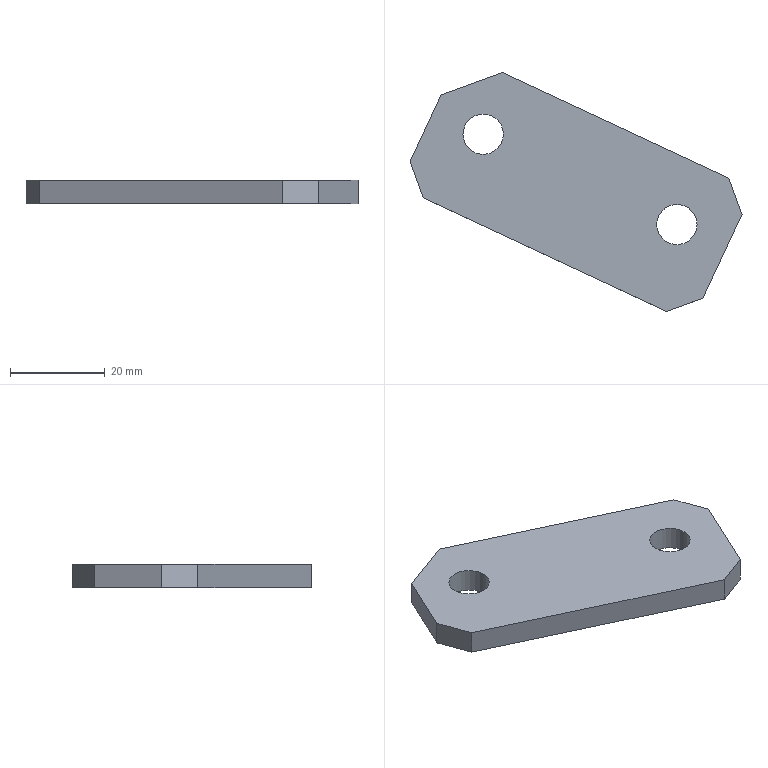Part | STEP file | gslz 2016.10.28-13_id1690_x_t | 1 solid | 12 faces | box 69.906 x 50.319 x 5 mm | volume 9493 mm3 | plane 10 | cylinder 2 | commonest cylinder face diameters 8.5 x2
STEP:
#1=CARTESIAN_POINT('',(0.,0.,0.));
#2=DIRECTION('',(0.,0.,1.));
#3=DIRECTION('',(1.,0.,0.));
#4=AXIS2_PLACEMENT_3D('',#1,#2,#3);
#5=CARTESIAN_POINT('',(735.517,61.885,-94.));
#6=VERTEX_POINT('',#5);
#7=CARTESIAN_POINT('',(728.93,47.759,-94.));
#8=VERTEX_POINT('',#7);
#9=CARTESIAN_POINT('',(744.057,80.199,-94.));
#10=DIRECTION('',(-0.4226,-0.9063,0.));
#11=VECTOR('',#10,1.);
#12=LINE('',#9,#11);
#13=CARTESIAN_POINT('',(744.057,80.199,-99.));
#14=DIRECTION('',(-0.9063,0.4226,0.));
#15=DIRECTION('',(-0.4226,-0.9063,0.));
#16=AXIS2_PLACEMENT_3D('',#13,#14,#15);
#17=PLANE('',#16);
#18=CARTESIAN_POINT('',(0.,5.));
#19=DIRECTION('',(1.,0.));
#20=VECTOR('',#19,1.);
#21=LINE('',#18,#20);
#22=(GEOMETRIC_REPRESENTATION_CONTEXT(2)PARAMETRIC_REPRESENTATION_CONTEXT()REPRESENTATION_CONTEXT('',''));
#23=DEFINITIONAL_REPRESENTATION('',(#21),#22);
#24=PCURVE('',#17,#23);
#25=CARTESIAN_POINT('',(-41.77,446.636,-94.));
#26=DIRECTION('',(0.,0.,-1.));
#27=DIRECTION('',(-1.,0.,0.));
#28=AXIS2_PLACEMENT_3D('',#25,#26,#27);
#29=PLANE('',#28);
#30=CARTESIAN_POINT('',(-785.827,-366.437));
#31=DIRECTION('',(0.4226,-0.9063));
#32=VECTOR('',#31,1.);
#33=LINE('',#30,#32);
#34=(GEOMETRIC_REPRESENTATION_CONTEXT(2)PARAMETRIC_REPRESENTATION_CONTEXT()REPRESENTATION_CONTEXT('',''));
#35=DEFINITIONAL_REPRESENTATION('',(#33),#34);
#36=PCURVE('',#29,#35);
#37=SURFACE_CURVE('',#12,(#24,#36),.PCURVE_S1.);
#38=EDGE_CURVE('',#6,#8,#37,.T.);
#39=ORIENTED_EDGE('',*,*,#38,.F.);
#40=CARTESIAN_POINT('',(735.517,61.885,-99.));
#41=VERTEX_POINT('',#40);
#42=CARTESIAN_POINT('',(735.517,61.885,-99.));
#43=DIRECTION('',(0.,0.,1.));
#44=VECTOR('',#43,1.);
#45=LINE('',#42,#44);
#46=CARTESIAN_POINT('',(20.207,0.));
#47=DIRECTION('',(0.,1.));
#48=VECTOR('',#47,1.);
#49=LINE('',#46,#48);
#50=(GEOMETRIC_REPRESENTATION_CONTEXT(2)PARAMETRIC_REPRESENTATION_CONTEXT()REPRESENTATION_CONTEXT('',''));
#51=DEFINITIONAL_REPRESENTATION('',(#49),#50);
#52=PCURVE('',#17,#51);
#53=CARTESIAN_POINT('',(172.812,-142.923,-99.));
#54=DIRECTION('',(0.342,-0.9397,0.));
#55=DIRECTION('',(0.9397,0.342,0.));
#56=AXIS2_PLACEMENT_3D('',#53,#54,#55);
#57=PLANE('',#56);
#58=CARTESIAN_POINT('',(598.818,0.));
#59=DIRECTION('',(0.,1.));
#60=VECTOR('',#59,1.);
#61=LINE('',#58,#60);
#62=(GEOMETRIC_REPRESENTATION_CONTEXT(2)PARAMETRIC_REPRESENTATION_CONTEXT()REPRESENTATION_CONTEXT('',''));
#63=DEFINITIONAL_REPRESENTATION('',(#61),#62);
#64=PCURVE('',#57,#63);
#65=SURFACE_CURVE('',#45,(#52,#64),.PCURVE_S1.);
#66=EDGE_CURVE('',#41,#6,#65,.T.);
#67=ORIENTED_EDGE('',*,*,#66,.F.);
#68=CARTESIAN_POINT('',(728.93,47.759,-99.));
#69=VERTEX_POINT('',#68);
#70=CARTESIAN_POINT('',(742.366,76.573,-99.));
#71=DIRECTION('',(-0.4226,-0.9063,0.));
#72=VECTOR('',#71,1.);
#73=LINE('',#70,#72);
#74=CARTESIAN_POINT('',(4.,0.));
#75=DIRECTION('',(1.,0.));
#76=VECTOR('',#75,1.);
#77=LINE('',#74,#76);
#78=(GEOMETRIC_REPRESENTATION_CONTEXT(2)PARAMETRIC_REPRESENTATION_CONTEXT()REPRESENTATION_CONTEXT('',''));
#79=DEFINITIONAL_REPRESENTATION('',(#77),#78);
#80=PCURVE('',#17,#79);
#81=CARTESIAN_POINT('',(-43.461,443.01,-99.));
#82=DIRECTION('',(0.,0.,-1.));
#83=DIRECTION('',(-1.,0.,0.));
#84=AXIS2_PLACEMENT_3D('',#81,#82,#83);
#85=PLANE('',#84);
#86=CARTESIAN_POINT('',(-785.827,-366.437));
#87=DIRECTION('',(0.4226,-0.9063));
#88=VECTOR('',#87,1.);
#89=LINE('',#86,#88);
#90=(GEOMETRIC_REPRESENTATION_CONTEXT(2)PARAMETRIC_REPRESENTATION_CONTEXT()REPRESENTATION_CONTEXT('',''));
#91=DEFINITIONAL_REPRESENTATION('',(#89),#90);
#92=PCURVE('',#85,#91);
#93=SURFACE_CURVE('',#73,(#80,#92),.PCURVE_S1.);
#94=EDGE_CURVE('',#41,#69,#93,.T.);
#95=ORIENTED_EDGE('',*,*,#94,.T.);
#96=CARTESIAN_POINT('',(728.93,47.759,-99.));
#97=DIRECTION('',(0.,0.,1.));
#98=VECTOR('',#97,1.);
#99=LINE('',#96,#98);
#100=CARTESIAN_POINT('',(35.793,0.));
#101=DIRECTION('',(0.,1.));
#102=VECTOR('',#101,1.);
#103=LINE('',#100,#102);
#104=(GEOMETRIC_REPRESENTATION_CONTEXT(2)PARAMETRIC_REPRESENTATION_CONTEXT()REPRESENTATION_CONTEXT('',''));
#105=DEFINITIONAL_REPRESENTATION('',(#103),#104);
#106=PCURVE('',#17,#105);
#107=CARTESIAN_POINT('',(511.546,645.016,-99.));
#108=DIRECTION('',(0.9397,0.342,0.));
#109=DIRECTION('',(-0.342,0.9397,0.));
#110=AXIS2_PLACEMENT_3D('',#107,#108,#109);
#111=PLANE('',#110);
#112=CARTESIAN_POINT('',(-635.588,0.));
#113=DIRECTION('',(0.,1.));
#114=VECTOR('',#113,1.);
#115=LINE('',#112,#114);
#116=(GEOMETRIC_REPRESENTATION_CONTEXT(2)PARAMETRIC_REPRESENTATION_CONTEXT()REPRESENTATION_CONTEXT('',''));
#117=DEFINITIONAL_REPRESENTATION('',(#115),#116);
#118=PCURVE('',#111,#117);
#119=SURFACE_CURVE('',#99,(#106,#118),.PCURVE_S1.);
#120=EDGE_CURVE('',#69,#8,#119,.T.);
#121=ORIENTED_EDGE('',*,*,#120,.T.);
#122=EDGE_LOOP('',(#39,#67,#95,#121));
#123=FACE_BOUND('',#122,.T.);
#124=ADVANCED_FACE('',(#123),#17,.T.);
#125=CARTESIAN_POINT('',(748.417,66.58,-94.));
#126=VERTEX_POINT('',#125);
#127=CARTESIAN_POINT('',(172.812,-142.923,-94.));
#128=DIRECTION('',(0.9397,0.342,0.));
#129=VECTOR('',#128,1.);
#130=LINE('',#127,#129);
#131=CARTESIAN_POINT('',(0.,5.));
#132=DIRECTION('',(1.,0.));
#133=VECTOR('',#132,1.);
#134=LINE('',#131,#133);
#135=(GEOMETRIC_REPRESENTATION_CONTEXT(2)PARAMETRIC_REPRESENTATION_CONTEXT()REPRESENTATION_CONTEXT('',''));
#136=DEFINITIONAL_REPRESENTATION('',(#134),#135);
#137=PCURVE('',#57,#136);
#138=CARTESIAN_POINT('',(-214.582,-589.559));
#139=DIRECTION('',(-0.9397,0.342));
#140=VECTOR('',#139,1.);
#141=LINE('',#138,#140);
#142=(GEOMETRIC_REPRESENTATION_CONTEXT(2)PARAMETRIC_REPRESENTATION_CONTEXT()REPRESENTATION_CONTEXT('',''));
#143=DEFINITIONAL_REPRESENTATION('',(#141),#142);
#144=PCURVE('',#29,#143);
#145=SURFACE_CURVE('',#130,(#137,#144),.PCURVE_S1.);
#146=EDGE_CURVE('',#6,#126,#145,.T.);
#147=ORIENTED_EDGE('',*,*,#146,.T.);
#148=CARTESIAN_POINT('',(748.417,66.58,-99.));
#149=VERTEX_POINT('',#148);
#150=CARTESIAN_POINT('',(748.417,66.58,-99.));
#151=DIRECTION('',(0.,0.,1.));
#152=VECTOR('',#151,1.);
#153=LINE('',#150,#152);
#154=CARTESIAN_POINT('',(612.546,0.));
#155=DIRECTION('',(0.,1.));
#156=VECTOR('',#155,1.);
#157=LINE('',#154,#156);
#158=(GEOMETRIC_REPRESENTATION_CONTEXT(2)PARAMETRIC_REPRESENTATION_CONTEXT()REPRESENTATION_CONTEXT('',''));
#159=DEFINITIONAL_REPRESENTATION('',(#157),#158);
#160=PCURVE('',#57,#159);
#161=CARTESIAN_POINT('',(-46.208,437.119,-99.));
#162=DIRECTION('',(-0.4226,-0.9063,0.));
#163=DIRECTION('',(0.9063,-0.4226,0.));
#164=AXIS2_PLACEMENT_3D('',#161,#162,#163);
#165=PLANE('',#164);
#166=CARTESIAN_POINT('',(876.771,0.));
#167=DIRECTION('',(0.,1.));
#168=VECTOR('',#167,1.);
#169=LINE('',#166,#168);
#170=(GEOMETRIC_REPRESENTATION_CONTEXT(2)PARAMETRIC_REPRESENTATION_CONTEXT()REPRESENTATION_CONTEXT('',''));
#171=DEFINITIONAL_REPRESENTATION('',(#169),#170);
#172=PCURVE('',#165,#171);
#173=SURFACE_CURVE('',#153,(#160,#172),.PCURVE_S1.);
#174=EDGE_CURVE('',#149,#126,#173,.T.);
#175=ORIENTED_EDGE('',*,*,#174,.F.);
#176=CARTESIAN_POINT('',(172.812,-142.923,-99.));
#177=DIRECTION('',(0.9397,0.342,0.));
#178=VECTOR('',#177,1.);
#179=LINE('',#176,#178);
#180=CARTESIAN_POINT('',(0.,0.));
#181=DIRECTION('',(1.,0.));
#182=VECTOR('',#181,1.);
#183=LINE('',#180,#182);
#184=(GEOMETRIC_REPRESENTATION_CONTEXT(2)PARAMETRIC_REPRESENTATION_CONTEXT()REPRESENTATION_CONTEXT('',''));
#185=DEFINITIONAL_REPRESENTATION('',(#183),#184);
#186=PCURVE('',#57,#185);
#187=CARTESIAN_POINT('',(-216.273,-585.934));
#188=DIRECTION('',(-0.9397,0.342));
#189=VECTOR('',#188,1.);
#190=LINE('',#187,#189);
#191=(GEOMETRIC_REPRESENTATION_CONTEXT(2)PARAMETRIC_REPRESENTATION_CONTEXT()REPRESENTATION_CONTEXT('',''));
#192=DEFINITIONAL_REPRESENTATION('',(#190),#191);
#193=PCURVE('',#85,#192);
#194=SURFACE_CURVE('',#179,(#186,#193),.PCURVE_S1.);
#195=EDGE_CURVE('',#41,#149,#194,.T.);
#196=ORIENTED_EDGE('',*,*,#195,.F.);
#197=ORIENTED_EDGE('',*,*,#66,.T.);
#198=EDGE_LOOP('',(#147,#175,#196,#197));
#199=FACE_BOUND('',#198,.T.);
#200=ADVANCED_FACE('',(#199),#57,.F.);
#201=CARTESIAN_POINT('',(796.076,44.356,-94.));
#202=VERTEX_POINT('',#201);
#203=CARTESIAN_POINT('',(-46.208,437.119,-94.));
#204=DIRECTION('',(0.9063,-0.4226,0.));
#205=VECTOR('',#204,1.);
#206=LINE('',#203,#205);
#207=CARTESIAN_POINT('',(0.,5.));
#208=DIRECTION('',(1.,0.));
#209=VECTOR('',#208,1.);
#210=LINE('',#207,#209);
#211=(GEOMETRIC_REPRESENTATION_CONTEXT(2)PARAMETRIC_REPRESENTATION_CONTEXT()REPRESENTATION_CONTEXT('',''));
#212=DEFINITIONAL_REPRESENTATION('',(#210),#211);
#213=PCURVE('',#165,#212);
#214=CARTESIAN_POINT('',(4.437,-9.516));
#215=DIRECTION('',(-0.9063,-0.4226));
#216=VECTOR('',#215,1.);
#217=LINE('',#214,#216);
#218=(GEOMETRIC_REPRESENTATION_CONTEXT(2)PARAMETRIC_REPRESENTATION_CONTEXT()REPRESENTATION_CONTEXT('',''));
#219=DEFINITIONAL_REPRESENTATION('',(#217),#218);
#220=PCURVE('',#29,#219);
#221=SURFACE_CURVE('',#206,(#213,#220),.PCURVE_S1.);
#222=EDGE_CURVE('',#126,#202,#221,.T.);
#223=ORIENTED_EDGE('',*,*,#222,.T.);
#224=CARTESIAN_POINT('',(796.076,44.356,-99.));
#225=VERTEX_POINT('',#224);
#226=CARTESIAN_POINT('',(796.076,44.356,-99.));
#227=DIRECTION('',(0.,0.,1.));
#228=VECTOR('',#227,1.);
#229=LINE('',#226,#228);
#230=CARTESIAN_POINT('',(929.357,0.));
#231=DIRECTION('',(0.,1.));
#232=VECTOR('',#231,1.);
#233=LINE('',#230,#232);
#234=(GEOMETRIC_REPRESENTATION_CONTEXT(2)PARAMETRIC_REPRESENTATION_CONTEXT()REPRESENTATION_CONTEXT('',''));
#235=DEFINITIONAL_REPRESENTATION('',(#233),#234);
#236=PCURVE('',#165,#235);
#237=CARTESIAN_POINT('',(568.776,668.857,-99.));
#238=DIRECTION('',(-0.9397,-0.342,0.));
#239=DIRECTION('',(0.342,-0.9397,0.));
#240=AXIS2_PLACEMENT_3D('',#237,#238,#239);
#241=PLANE('',#240);
#242=CARTESIAN_POINT('',(664.579,0.));
#243=DIRECTION('',(0.,1.));
#244=VECTOR('',#243,1.);
#245=LINE('',#242,#244);
#246=(GEOMETRIC_REPRESENTATION_CONTEXT(2)PARAMETRIC_REPRESENTATION_CONTEXT()REPRESENTATION_CONTEXT('',''));
#247=DEFINITIONAL_REPRESENTATION('',(#245),#246);
#248=PCURVE('',#241,#247);
#249=SURFACE_CURVE('',#229,(#236,#248),.PCURVE_S1.);
#250=EDGE_CURVE('',#225,#202,#249,.T.);
#251=ORIENTED_EDGE('',*,*,#250,.F.);
#252=CARTESIAN_POINT('',(-46.208,437.119,-99.));
#253=DIRECTION('',(0.9063,-0.4226,0.));
#254=VECTOR('',#253,1.);
#255=LINE('',#252,#254);
#256=CARTESIAN_POINT('',(0.,0.));
#257=DIRECTION('',(1.,0.));
#258=VECTOR('',#257,1.);
#259=LINE('',#256,#258);
#260=(GEOMETRIC_REPRESENTATION_CONTEXT(2)PARAMETRIC_REPRESENTATION_CONTEXT()REPRESENTATION_CONTEXT('',''));
#261=DEFINITIONAL_REPRESENTATION('',(#259),#260);
#262=PCURVE('',#165,#261);
#263=CARTESIAN_POINT('',(2.747,-5.891));
#264=DIRECTION('',(-0.9063,-0.4226));
#265=VECTOR('',#264,1.);
#266=LINE('',#263,#265);
#267=(GEOMETRIC_REPRESENTATION_CONTEXT(2)PARAMETRIC_REPRESENTATION_CONTEXT()REPRESENTATION_CONTEXT('',''));
#268=DEFINITIONAL_REPRESENTATION('',(#266),#267);
#269=PCURVE('',#85,#268);
#270=SURFACE_CURVE('',#255,(#262,#269),.PCURVE_S1.);
#271=EDGE_CURVE('',#149,#225,#270,.T.);
#272=ORIENTED_EDGE('',*,*,#271,.F.);
#273=ORIENTED_EDGE('',*,*,#174,.T.);
#274=EDGE_LOOP('',(#223,#251,#272,#273));
#275=FACE_BOUND('',#274,.T.);
#276=ADVANCED_FACE('',(#275),#165,.F.);
#277=CARTESIAN_POINT('',(798.836,36.772,-94.));
#278=VERTEX_POINT('',#277);
#279=CARTESIAN_POINT('',(568.776,668.857,-94.));
#280=DIRECTION('',(0.342,-0.9397,0.));
#281=VECTOR('',#280,1.);
#282=LINE('',#279,#281);
#283=CARTESIAN_POINT('',(0.,5.));
#284=DIRECTION('',(1.,0.));
#285=VECTOR('',#284,1.);
#286=LINE('',#283,#285);
#287=(GEOMETRIC_REPRESENTATION_CONTEXT(2)PARAMETRIC_REPRESENTATION_CONTEXT()REPRESENTATION_CONTEXT('',''));
#288=DEFINITIONAL_REPRESENTATION('',(#286),#287);
#289=PCURVE('',#241,#288);
#290=CARTESIAN_POINT('',(-610.546,222.221));
#291=DIRECTION('',(-0.342,-0.9397));
#292=VECTOR('',#291,1.);
#293=LINE('',#290,#292);
#294=(GEOMETRIC_REPRESENTATION_CONTEXT(2)PARAMETRIC_REPRESENTATION_CONTEXT()REPRESENTATION_CONTEXT('',''));
#295=DEFINITIONAL_REPRESENTATION('',(#293),#294);
#296=PCURVE('',#29,#295);
#297=SURFACE_CURVE('',#282,(#289,#296),.PCURVE_S1.);
#298=EDGE_CURVE('',#202,#278,#297,.T.);
#299=ORIENTED_EDGE('',*,*,#298,.T.);
#300=CARTESIAN_POINT('',(798.836,36.772,-99.));
#301=VERTEX_POINT('',#300);
#302=CARTESIAN_POINT('',(798.836,36.772,-99.));
#303=DIRECTION('',(0.,0.,1.));
#304=VECTOR('',#303,1.);
#305=LINE('',#302,#304);
#306=CARTESIAN_POINT('',(672.65,0.));
#307=DIRECTION('',(0.,1.));
#308=VECTOR('',#307,1.);
#309=LINE('',#306,#308);
#310=(GEOMETRIC_REPRESENTATION_CONTEXT(2)PARAMETRIC_REPRESENTATION_CONTEXT()REPRESENTATION_CONTEXT('',''));
#311=DEFINITIONAL_REPRESENTATION('',(#309),#310);
#312=PCURVE('',#241,#311);
#313=CARTESIAN_POINT('',(805.686,51.461,-99.));
#314=DIRECTION('',(-0.9063,0.4226,0.));
#315=DIRECTION('',(-0.4226,-0.9063,0.));
#316=AXIS2_PLACEMENT_3D('',#313,#314,#315);
#317=PLANE('',#316);
#318=CARTESIAN_POINT('',(16.207,0.));
#319=DIRECTION('',(0.,1.));
#320=VECTOR('',#319,1.);
#321=LINE('',#318,#320);
#322=(GEOMETRIC_REPRESENTATION_CONTEXT(2)PARAMETRIC_REPRESENTATION_CONTEXT()REPRESENTATION_CONTEXT('',''));
#323=DEFINITIONAL_REPRESENTATION('',(#321),#322);
#324=PCURVE('',#317,#323);
#325=SURFACE_CURVE('',#305,(#312,#324),.PCURVE_S1.);
#326=EDGE_CURVE('',#301,#278,#325,.T.);
#327=ORIENTED_EDGE('',*,*,#326,.F.);
#328=CARTESIAN_POINT('',(568.776,668.857,-99.));
#329=DIRECTION('',(0.342,-0.9397,0.));
#330=VECTOR('',#329,1.);
#331=LINE('',#328,#330);
#332=CARTESIAN_POINT('',(0.,0.));
#333=DIRECTION('',(1.,0.));
#334=VECTOR('',#333,1.);
#335=LINE('',#332,#334);
#336=(GEOMETRIC_REPRESENTATION_CONTEXT(2)PARAMETRIC_REPRESENTATION_CONTEXT()REPRESENTATION_CONTEXT('',''));
#337=DEFINITIONAL_REPRESENTATION('',(#335),#336);
#338=PCURVE('',#241,#337);
#339=CARTESIAN_POINT('',(-612.237,225.846));
#340=DIRECTION('',(-0.342,-0.9397));
#341=VECTOR('',#340,1.);
#342=LINE('',#339,#341);
#343=(GEOMETRIC_REPRESENTATION_CONTEXT(2)PARAMETRIC_REPRESENTATION_CONTEXT()REPRESENTATION_CONTEXT('',''));
#344=DEFINITIONAL_REPRESENTATION('',(#342),#343);
#345=PCURVE('',#85,#344);
#346=SURFACE_CURVE('',#331,(#338,#345),.PCURVE_S1.);
#347=EDGE_CURVE('',#225,#301,#346,.T.);
#348=ORIENTED_EDGE('',*,*,#347,.F.);
#349=ORIENTED_EDGE('',*,*,#250,.T.);
#350=EDGE_LOOP('',(#299,#327,#348,#349));
#351=FACE_BOUND('',#350,.T.);
#352=ADVANCED_FACE('',(#351),#241,.F.);
#353=CARTESIAN_POINT('',(790.559,19.021,-94.));
#354=VERTEX_POINT('',#353);
#355=CARTESIAN_POINT('',(805.686,51.461,-94.));
#356=DIRECTION('',(-0.4226,-0.9063,0.));
#357=VECTOR('',#356,1.);
#358=LINE('',#355,#357);
#359=CARTESIAN_POINT('',(0.,5.));
#360=DIRECTION('',(1.,0.));
#361=VECTOR('',#360,1.);
#362=LINE('',#359,#361);
#363=(GEOMETRIC_REPRESENTATION_CONTEXT(2)PARAMETRIC_REPRESENTATION_CONTEXT()REPRESENTATION_CONTEXT('',''));
#364=DEFINITIONAL_REPRESENTATION('',(#362),#363);
#365=PCURVE('',#317,#364);
#366=CARTESIAN_POINT('',(-847.456,-395.175));
#367=DIRECTION('',(0.4226,-0.9063));
#368=VECTOR('',#367,1.);
#369=LINE('',#366,#368);
#370=(GEOMETRIC_REPRESENTATION_CONTEXT(2)PARAMETRIC_REPRESENTATION_CONTEXT()REPRESENTATION_CONTEXT('',''));
#371=DEFINITIONAL_REPRESENTATION('',(#369),#370);
#372=PCURVE('',#29,#371);
#373=SURFACE_CURVE('',#358,(#365,#372),.PCURVE_S1.);
#374=EDGE_CURVE('',#278,#354,#373,.T.);
#375=ORIENTED_EDGE('',*,*,#374,.T.);
#376=CARTESIAN_POINT('',(790.559,19.021,-99.));
#377=VERTEX_POINT('',#376);
#378=CARTESIAN_POINT('',(790.559,19.021,-99.));
#379=DIRECTION('',(0.,0.,1.));
#380=VECTOR('',#379,1.);
#381=LINE('',#378,#380);
#382=CARTESIAN_POINT('',(35.793,0.));
#383=DIRECTION('',(0.,1.));
#384=VECTOR('',#383,1.);
#385=LINE('',#382,#384);
#386=(GEOMETRIC_REPRESENTATION_CONTEXT(2)PARAMETRIC_REPRESENTATION_CONTEXT()REPRESENTATION_CONTEXT('',''));
#387=DEFINITIONAL_REPRESENTATION('',(#385),#386);
#388=PCURVE('',#317,#387);
#389=CARTESIAN_POINT('',(190.369,-199.43,-99.));
#390=DIRECTION('',(-0.342,0.9397,0.));
#391=DIRECTION('',(-0.9397,-0.342,0.));
#392=AXIS2_PLACEMENT_3D('',#389,#390,#391);
#393=PLANE('',#392);
#394=CARTESIAN_POINT('',(-638.709,0.));
#395=DIRECTION('',(0.,1.));
#396=VECTOR('',#395,1.);
#397=LINE('',#394,#396);
#398=(GEOMETRIC_REPRESENTATION_CONTEXT(2)PARAMETRIC_REPRESENTATION_CONTEXT()REPRESENTATION_CONTEXT('',''));
#399=DEFINITIONAL_REPRESENTATION('',(#397),#398);
#400=PCURVE('',#393,#399);
#401=SURFACE_CURVE('',#381,(#388,#400),.PCURVE_S1.);
#402=EDGE_CURVE('',#377,#354,#401,.T.);
#403=ORIENTED_EDGE('',*,*,#402,.F.);
#404=CARTESIAN_POINT('',(803.995,47.835,-99.));
#405=DIRECTION('',(-0.4226,-0.9063,0.));
#406=VECTOR('',#405,1.);
#407=LINE('',#404,#406);
#408=CARTESIAN_POINT('',(4.,0.));
#409=DIRECTION('',(1.,0.));
#410=VECTOR('',#409,1.);
#411=LINE('',#408,#410);
#412=(GEOMETRIC_REPRESENTATION_CONTEXT(2)PARAMETRIC_REPRESENTATION_CONTEXT()REPRESENTATION_CONTEXT('',''));
#413=DEFINITIONAL_REPRESENTATION('',(#411),#412);
#414=PCURVE('',#317,#413);
#415=CARTESIAN_POINT('',(-847.456,-395.175));
#416=DIRECTION('',(0.4226,-0.9063));
#417=VECTOR('',#416,1.);
#418=LINE('',#415,#417);
#419=(GEOMETRIC_REPRESENTATION_CONTEXT(2)PARAMETRIC_REPRESENTATION_CONTEXT()REPRESENTATION_CONTEXT('',''));
#420=DEFINITIONAL_REPRESENTATION('',(#418),#419);
#421=PCURVE('',#85,#420);
#422=SURFACE_CURVE('',#407,(#414,#421),.PCURVE_S1.);
#423=EDGE_CURVE('',#301,#377,#422,.T.);
#424=ORIENTED_EDGE('',*,*,#423,.F.);
#425=ORIENTED_EDGE('',*,*,#326,.T.);
#426=EDGE_LOOP('',(#375,#403,#424,#425));
#427=FACE_BOUND('',#426,.T.);
#428=ADVANCED_FACE('',(#427),#317,.F.);
#429=CARTESIAN_POINT('',(782.975,16.261,-94.));
#430=VERTEX_POINT('',#429);
#431=CARTESIAN_POINT('',(190.369,-199.43,-94.));
#432=DIRECTION('',(-0.9397,-0.342,0.));
#433=VECTOR('',#432,1.);
#434=LINE('',#431,#433);
#435=CARTESIAN_POINT('',(0.,5.));
#436=DIRECTION('',(1.,0.));
#437=VECTOR('',#436,1.);
#438=LINE('',#435,#437);
#439=(GEOMETRIC_REPRESENTATION_CONTEXT(2)PARAMETRIC_REPRESENTATION_CONTEXT()REPRESENTATION_CONTEXT('',''));
#440=DEFINITIONAL_REPRESENTATION('',(#438),#439);
#441=PCURVE('',#393,#440);
#442=CARTESIAN_POINT('',(-232.139,-646.066));
#443=DIRECTION('',(0.9397,-0.342));
#444=VECTOR('',#443,1.);
#445=LINE('',#442,#444);
#446=(GEOMETRIC_REPRESENTATION_CONTEXT(2)PARAMETRIC_REPRESENTATION_CONTEXT()REPRESENTATION_CONTEXT('',''));
#447=DEFINITIONAL_REPRESENTATION('',(#445),#446);
#448=PCURVE('',#29,#447);
#449=SURFACE_CURVE('',#434,(#441,#448),.PCURVE_S1.);
#450=EDGE_CURVE('',#354,#430,#449,.T.);
#451=ORIENTED_EDGE('',*,*,#450,.T.);
#452=CARTESIAN_POINT('',(782.975,16.261,-99.));
#453=VERTEX_POINT('',#452);
#454=CARTESIAN_POINT('',(782.975,16.261,-99.));
#455=DIRECTION('',(0.,0.,1.));
#456=VECTOR('',#455,1.);
#457=LINE('',#454,#456);
#458=CARTESIAN_POINT('',(-630.638,0.));
#459=DIRECTION('',(0.,1.));
#460=VECTOR('',#459,1.);
#461=LINE('',#458,#460);
#462=(GEOMETRIC_REPRESENTATION_CONTEXT(2)PARAMETRIC_REPRESENTATION_CONTEXT()REPRESENTATION_CONTEXT('',''));
#463=DEFINITIONAL_REPRESENTATION('',(#461),#462);
#464=PCURVE('',#393,#463);
#465=CARTESIAN_POINT('',(-1466.318,1065.122,-99.));
#466=DIRECTION('',(-0.4226,-0.9063,0.));
#467=DIRECTION('',(0.9063,-0.4226,0.));
#468=AXIS2_PLACEMENT_3D('',#465,#466,#467);
#469=PLANE('',#468);
#470=CARTESIAN_POINT('',(2481.819,0.));
#471=DIRECTION('',(0.,1.));
#472=VECTOR('',#471,1.);
#473=LINE('',#470,#472);
#474=(GEOMETRIC_REPRESENTATION_CONTEXT(2)PARAMETRIC_REPRESENTATION_CONTEXT()REPRESENTATION_CONTEXT('',''));
#475=DEFINITIONAL_REPRESENTATION('',(#473),#474);
#476=PCURVE('',#469,#475);
#477=SURFACE_CURVE('',#457,(#464,#476),.PCURVE_S1.);
#478=EDGE_CURVE('',#453,#430,#477,.T.);
#479=ORIENTED_EDGE('',*,*,#478,.F.);
#480=CARTESIAN_POINT('',(190.369,-199.43,-99.));
#481=DIRECTION('',(-0.9397,-0.342,0.));
#482=VECTOR('',#481,1.);
#483=LINE('',#480,#482);
#484=CARTESIAN_POINT('',(0.,0.));
#485=DIRECTION('',(1.,0.));
#486=VECTOR('',#485,1.);
#487=LINE('',#484,#486);
#488=(GEOMETRIC_REPRESENTATION_CONTEXT(2)PARAMETRIC_REPRESENTATION_CONTEXT()REPRESENTATION_CONTEXT('',''));
#489=DEFINITIONAL_REPRESENTATION('',(#487),#488);
#490=PCURVE('',#393,#489);
#491=CARTESIAN_POINT('',(-233.83,-642.441));
#492=DIRECTION('',(0.9397,-0.342));
#493=VECTOR('',#492,1.);
#494=LINE('',#491,#493);
#495=(GEOMETRIC_REPRESENTATION_CONTEXT(2)PARAMETRIC_REPRESENTATION_CONTEXT()REPRESENTATION_CONTEXT('',''));
#496=DEFINITIONAL_REPRESENTATION('',(#494),#495);
#497=PCURVE('',#85,#496);
#498=SURFACE_CURVE('',#483,(#490,#497),.PCURVE_S1.);
#499=EDGE_CURVE('',#377,#453,#498,.T.);
#500=ORIENTED_EDGE('',*,*,#499,.F.);
#501=ORIENTED_EDGE('',*,*,#402,.T.);
#502=EDGE_LOOP('',(#451,#479,#500,#501));
#503=FACE_BOUND('',#502,.T.);
#504=ADVANCED_FACE('',(#503),#393,.F.);
#505=CARTESIAN_POINT('',(731.691,40.175,-94.));
#506=VERTEX_POINT('',#505);
#507=CARTESIAN_POINT('',(-1466.318,1065.122,-94.));
#508=DIRECTION('',(0.9063,-0.4226,0.));
#509=VECTOR('',#508,1.);
#510=LINE('',#507,#509);
#511=CARTESIAN_POINT('',(0.,5.));
#512=DIRECTION('',(1.,0.));
#513=VECTOR('',#512,1.);
#514=LINE('',#511,#513);
#515=(GEOMETRIC_REPRESENTATION_CONTEXT(2)PARAMETRIC_REPRESENTATION_CONTEXT()REPRESENTATION_CONTEXT('',''));
#516=DEFINITIONAL_REPRESENTATION('',(#514),#515);
#517=PCURVE('',#469,#516);
#518=CARTESIAN_POINT('',(1424.547,618.487));
#519=DIRECTION('',(-0.9063,-0.4226));
#520=VECTOR('',#519,1.);
#521=LINE('',#518,#520);
#522=(GEOMETRIC_REPRESENTATION_CONTEXT(2)PARAMETRIC_REPRESENTATION_CONTEXT()REPRESENTATION_CONTEXT('',''));
#523=DEFINITIONAL_REPRESENTATION('',(#521),#522);
#524=PCURVE('',#29,#523);
#525=SURFACE_CURVE('',#510,(#517,#524),.PCURVE_S1.);
#526=EDGE_CURVE('',#506,#430,#525,.T.);
#527=ORIENTED_EDGE('',*,*,#526,.F.);
#528=CARTESIAN_POINT('',(731.691,40.175,-99.));
#529=VERTEX_POINT('',#528);
#530=CARTESIAN_POINT('',(731.691,40.175,-99.));
#531=DIRECTION('',(0.,0.,1.));
#532=VECTOR('',#531,1.);
#533=LINE('',#530,#532);
#534=CARTESIAN_POINT('',(2425.233,0.));
#535=DIRECTION('',(0.,1.));
#536=VECTOR('',#535,1.);
#537=LINE('',#534,#536);
#538=(GEOMETRIC_REPRESENTATION_CONTEXT(2)PARAMETRIC_REPRESENTATION_CONTEXT()REPRESENTATION_CONTEXT('',''));
#539=DEFINITIONAL_REPRESENTATION('',(#537),#538);
#540=PCURVE('',#469,#539);
#541=CARTESIAN_POINT('',(-643.659,0.));
#542=DIRECTION('',(0.,1.));
#543=VECTOR('',#542,1.);
#544=LINE('',#541,#543);
#545=(GEOMETRIC_REPRESENTATION_CONTEXT(2)PARAMETRIC_REPRESENTATION_CONTEXT()REPRESENTATION_CONTEXT('',''));
#546=DEFINITIONAL_REPRESENTATION('',(#544),#545);
#547=PCURVE('',#111,#546);
#548=SURFACE_CURVE('',#533,(#540,#547),.PCURVE_S1.);
#549=EDGE_CURVE('',#529,#506,#548,.T.);
#550=ORIENTED_EDGE('',*,*,#549,.F.);
#551=CARTESIAN_POINT('',(-1466.318,1065.122,-99.));
#552=DIRECTION('',(0.9063,-0.4226,0.));
#553=VECTOR('',#552,1.);
#554=LINE('',#551,#553);
#555=CARTESIAN_POINT('',(0.,0.));
#556=DIRECTION('',(1.,0.));
#557=VECTOR('',#556,1.);
#558=LINE('',#555,#557);
#559=(GEOMETRIC_REPRESENTATION_CONTEXT(2)PARAMETRIC_REPRESENTATION_CONTEXT()REPRESENTATION_CONTEXT('',''));
#560=DEFINITIONAL_REPRESENTATION('',(#558),#559);
#561=PCURVE('',#469,#560);
#562=CARTESIAN_POINT('',(1422.857,622.112));
#563=DIRECTION('',(-0.9063,-0.4226));
#564=VECTOR('',#563,1.);
#565=LINE('',#562,#564);
#566=(GEOMETRIC_REPRESENTATION_CONTEXT(2)PARAMETRIC_REPRESENTATION_CONTEXT()REPRESENTATION_CONTEXT('',''));
#567=DEFINITIONAL_REPRESENTATION('',(#565),#566);
#568=PCURVE('',#85,#567);
#569=SURFACE_CURVE('',#554,(#561,#568),.PCURVE_S1.);
#570=EDGE_CURVE('',#529,#453,#569,.T.);
#571=ORIENTED_EDGE('',*,*,#570,.T.);
#572=ORIENTED_EDGE('',*,*,#478,.T.);
#573=EDGE_LOOP('',(#527,#550,#571,#572));
#574=FACE_BOUND('',#573,.T.);
#575=ADVANCED_FACE('',(#574),#469,.T.);
#576=CARTESIAN_POINT('',(511.546,645.016,-94.));
#577=DIRECTION('',(-0.342,0.9397,0.));
#578=VECTOR('',#577,1.);
#579=LINE('',#576,#578);
#580=CARTESIAN_POINT('',(0.,5.));
#581=DIRECTION('',(1.,0.));
#582=VECTOR('',#581,1.);
#583=LINE('',#580,#582);
#584=(GEOMETRIC_REPRESENTATION_CONTEXT(2)PARAMETRIC_REPRESENTATION_CONTEXT()REPRESENTATION_CONTEXT('',''));
#585=DEFINITIONAL_REPRESENTATION('',(#583),#584);
#586=PCURVE('',#111,#585);
#587=CARTESIAN_POINT('',(-553.316,198.381));
#588=DIRECTION('',(0.342,0.9397));
#589=VECTOR('',#588,1.);
#590=LINE('',#587,#589);
#591=(GEOMETRIC_REPRESENTATION_CONTEXT(2)PARAMETRIC_REPRESENTATION_CONTEXT()REPRESENTATION_CONTEXT('',''));
#592=DEFINITIONAL_REPRESENTATION('',(#590),#591);
#593=PCURVE('',#29,#592);
#594=SURFACE_CURVE('',#579,(#586,#593),.PCURVE_S1.);
#595=EDGE_CURVE('',#506,#8,#594,.T.);
#596=ORIENTED_EDGE('',*,*,#595,.T.);
#597=ORIENTED_EDGE('',*,*,#120,.F.);
#598=CARTESIAN_POINT('',(511.546,645.016,-99.));
#599=DIRECTION('',(-0.342,0.9397,0.));
#600=VECTOR('',#599,1.);
#601=LINE('',#598,#600);
#602=CARTESIAN_POINT('',(0.,0.));
#603=DIRECTION('',(1.,0.));
#604=VECTOR('',#603,1.);
#605=LINE('',#602,#604);
#606=(GEOMETRIC_REPRESENTATION_CONTEXT(2)PARAMETRIC_REPRESENTATION_CONTEXT()REPRESENTATION_CONTEXT('',''));
#607=DEFINITIONAL_REPRESENTATION('',(#605),#606);
#608=PCURVE('',#111,#607);
#609=CARTESIAN_POINT('',(-555.007,202.006));
#610=DIRECTION('',(0.342,0.9397));
#611=VECTOR('',#610,1.);
#612=LINE('',#609,#611);
#613=(GEOMETRIC_REPRESENTATION_CONTEXT(2)PARAMETRIC_REPRESENTATION_CONTEXT()REPRESENTATION_CONTEXT('',''));
#614=DEFINITIONAL_REPRESENTATION('',(#612),#613);
#615=PCURVE('',#85,#614);
#616=SURFACE_CURVE('',#601,(#608,#615),.PCURVE_S1.);
#617=EDGE_CURVE('',#529,#69,#616,.T.);
#618=ORIENTED_EDGE('',*,*,#617,.F.);
#619=ORIENTED_EDGE('',*,*,#549,.T.);
#620=EDGE_LOOP('',(#596,#597,#618,#619));
#621=FACE_BOUND('',#620,.T.);
#622=ADVANCED_FACE('',(#621),#111,.F.);
#623=CARTESIAN_POINT('',(780.87,34.569,-99.));
#624=VERTEX_POINT('',#623);
#625=CARTESIAN_POINT('',(785.12,34.569,-99.));
#626=DIRECTION('',(0.,0.,-1.));
#627=DIRECTION('',(-1.,0.,0.));
#628=AXIS2_PLACEMENT_3D('',#625,#626,#627);
#629=CIRCLE('',#628,4.25);
#630=CARTESIAN_POINT('',(785.12,34.569,-99.));
#631=DIRECTION('',(0.,0.,1.));
#632=DIRECTION('',(1.,0.,0.));
#633=AXIS2_PLACEMENT_3D('',#630,#631,#632);
#634=CYLINDRICAL_SURFACE('',#633,4.25);
#635=CARTESIAN_POINT('',(9.425,0.));
#636=DIRECTION('',(-1.,0.));
#637=VECTOR('',#636,1.);
#638=LINE('',#635,#637);
#639=(GEOMETRIC_REPRESENTATION_CONTEXT(2)PARAMETRIC_REPRESENTATION_CONTEXT()REPRESENTATION_CONTEXT('',''));
#640=DEFINITIONAL_REPRESENTATION('',(#638),#639);
#641=PCURVE('',#634,#640);
#642=CARTESIAN_POINT('',(-828.581,-408.441));
#643=DIRECTION('',(1.,0.));
#644=AXIS2_PLACEMENT_2D('',#642,#643);
#645=CIRCLE('',#644,4.25);
#646=(GEOMETRIC_REPRESENTATION_CONTEXT(2)PARAMETRIC_REPRESENTATION_CONTEXT()REPRESENTATION_CONTEXT('',''));
#647=DEFINITIONAL_REPRESENTATION('',(#645),#646);
#648=PCURVE('',#85,#647);
#649=SURFACE_CURVE('',#629,(#641,#648),.PCURVE_S1.);
#650=EDGE_CURVE('',#624,#624,#649,.T.);
#651=ORIENTED_EDGE('',*,*,#650,.F.);
#652=CARTESIAN_POINT('',(780.87,34.569,-94.));
#653=VERTEX_POINT('',#652);
#654=CARTESIAN_POINT('',(780.87,34.569,-99.));
#655=CARTESIAN_POINT('',(780.87,34.569,-94.));
#656=B_SPLINE_CURVE_WITH_KNOTS('',1,(#654,#655),.UNSPECIFIED.,.F.,.F.,(2,2),(0.,5.),.PIECEWISE_BEZIER_KNOTS.);
#657=CARTESIAN_POINT('',(9.425,0.));
#658=DIRECTION('',(0.,1.));
#659=VECTOR('',#658,1.);
#660=LINE('',#657,#659);
#661=(GEOMETRIC_REPRESENTATION_CONTEXT(2)PARAMETRIC_REPRESENTATION_CONTEXT()REPRESENTATION_CONTEXT('',''));
#662=DEFINITIONAL_REPRESENTATION('',(#660),#661);
#663=PCURVE('',#634,#662);
#664=CARTESIAN_POINT('',(3.142,0.));
#665=DIRECTION('',(0.,1.));
#666=VECTOR('',#665,1.);
#667=LINE('',#664,#666);
#668=(GEOMETRIC_REPRESENTATION_CONTEXT(2)PARAMETRIC_REPRESENTATION_CONTEXT()REPRESENTATION_CONTEXT('',''));
#669=DEFINITIONAL_REPRESENTATION('',(#667),#668);
#670=PCURVE('',#634,#669);
#671=SEAM_CURVE('',#656,(#663,#670),.PCURVE_S1.);
#672=EDGE_CURVE('',#624,#653,#671,.T.);
#673=ORIENTED_EDGE('',*,*,#672,.T.);
#674=CARTESIAN_POINT('',(785.12,34.569,-94.));
#675=DIRECTION('',(0.,0.,-1.));
#676=DIRECTION('',(-1.,0.,0.));
#677=AXIS2_PLACEMENT_3D('',#674,#675,#676);
#678=CIRCLE('',#677,4.25);
#679=CARTESIAN_POINT('',(9.425,5.));
#680=DIRECTION('',(-1.,0.));
#681=VECTOR('',#680,1.);
#682=LINE('',#679,#681);
#683=(GEOMETRIC_REPRESENTATION_CONTEXT(2)PARAMETRIC_REPRESENTATION_CONTEXT()REPRESENTATION_CONTEXT('',''));
#684=DEFINITIONAL_REPRESENTATION('',(#682),#683);
#685=PCURVE('',#634,#684);
#686=CARTESIAN_POINT('',(-826.891,-412.066));
#687=DIRECTION('',(1.,0.));
#688=AXIS2_PLACEMENT_2D('',#686,#687);
#689=CIRCLE('',#688,4.25);
#690=(GEOMETRIC_REPRESENTATION_CONTEXT(2)PARAMETRIC_REPRESENTATION_CONTEXT()REPRESENTATION_CONTEXT('',''));
#691=DEFINITIONAL_REPRESENTATION('',(#689),#690);
#692=PCURVE('',#29,#691);
#693=SURFACE_CURVE('',#678,(#685,#692),.PCURVE_S1.);
#694=EDGE_CURVE('',#653,#653,#693,.T.);
#695=ORIENTED_EDGE('',*,*,#694,.T.);
#696=ORIENTED_EDGE('',*,*,#672,.F.);
#697=EDGE_LOOP('',(#651,#673,#695,#696));
#698=FACE_BOUND('',#697,.F.);
#699=ADVANCED_FACE('',(#698),#634,.F.);
#700=CARTESIAN_POINT('',(740.087,53.587,-99.));
#701=VERTEX_POINT('',#700);
#702=CARTESIAN_POINT('',(744.337,53.587,-99.));
#703=DIRECTION('',(0.,0.,1.));
#704=DIRECTION('',(-1.,0.,0.));
#705=AXIS2_PLACEMENT_3D('',#702,#703,#704);
#706=CIRCLE('',#705,4.25);
#707=CARTESIAN_POINT('',(744.337,53.587,-99.));
#708=DIRECTION('',(0.,0.,1.));
#709=DIRECTION('',(1.,0.,0.));
#710=AXIS2_PLACEMENT_3D('',#707,#708,#709);
#711=CYLINDRICAL_SURFACE('',#710,4.25);
#712=CARTESIAN_POINT('',(3.142,0.));
#713=DIRECTION('',(1.,0.));
#714=VECTOR('',#713,1.);
#715=LINE('',#712,#714);
#716=(GEOMETRIC_REPRESENTATION_CONTEXT(2)PARAMETRIC_REPRESENTATION_CONTEXT()REPRESENTATION_CONTEXT('',''));
#717=DEFINITIONAL_REPRESENTATION('',(#715),#716);
#718=PCURVE('',#711,#717);
#719=CARTESIAN_POINT('',(-783.547,-389.423));
#720=CARTESIAN_POINT('',(-783.547,-396.784));
#721=CARTESIAN_POINT('',(-789.922,-393.104));
#722=CARTESIAN_POINT('',(-796.297,-389.423));
#723=CARTESIAN_POINT('',(-789.922,-385.743));
#724=CARTESIAN_POINT('',(-783.547,-382.062));
#725=CARTESIAN_POINT('',(-783.547,-389.423));
#726=(BOUNDED_CURVE()B_SPLINE_CURVE(2,(#719,#720,#721,#722,#723,#724,#725),.UNSPECIFIED.,.T.,.F.)B_SPLINE_CURVE_WITH_KNOTS((1,2,2,2,2,1),(-2.094,0.,2.094,4.189,6.283,8.378),.UNSPECIFIED.)CURVE()GEOMETRIC_REPRESENTATION_ITEM()RATIONAL_B_SPLINE_CURVE((1.,0.5,1.,0.5,1.,0.5,1.))REPRESENTATION_ITEM(''));
#727=(GEOMETRIC_REPRESENTATION_CONTEXT(2)PARAMETRIC_REPRESENTATION_CONTEXT()REPRESENTATION_CONTEXT('',''));
#728=DEFINITIONAL_REPRESENTATION('',(#726),#727);
#729=PCURVE('',#85,#728);
#730=SURFACE_CURVE('',#706,(#718,#729),.PCURVE_S1.);
#731=EDGE_CURVE('',#701,#701,#730,.T.);
#732=ORIENTED_EDGE('',*,*,#731,.T.);
#733=CARTESIAN_POINT('',(740.087,53.587,-94.));
#734=VERTEX_POINT('',#733);
#735=CARTESIAN_POINT('',(740.087,53.587,-99.));
#736=CARTESIAN_POINT('',(740.087,53.587,-94.));
#737=B_SPLINE_CURVE_WITH_KNOTS('',1,(#735,#736),.UNSPECIFIED.,.F.,.F.,(2,2),(0.,5.),.PIECEWISE_BEZIER_KNOTS.);
#738=CARTESIAN_POINT('',(9.425,0.));
#739=DIRECTION('',(0.,1.));
#740=VECTOR('',#739,1.);
#741=LINE('',#738,#740);
#742=(GEOMETRIC_REPRESENTATION_CONTEXT(2)PARAMETRIC_REPRESENTATION_CONTEXT()REPRESENTATION_CONTEXT('',''));
#743=DEFINITIONAL_REPRESENTATION('',(#741),#742);
#744=PCURVE('',#711,#743);
#745=CARTESIAN_POINT('',(3.142,0.));
#746=DIRECTION('',(0.,1.));
#747=VECTOR('',#746,1.);
#748=LINE('',#745,#747);
#749=(GEOMETRIC_REPRESENTATION_CONTEXT(2)PARAMETRIC_REPRESENTATION_CONTEXT()REPRESENTATION_CONTEXT('',''));
#750=DEFINITIONAL_REPRESENTATION('',(#748),#749);
#751=PCURVE('',#711,#750);
#752=SEAM_CURVE('',#737,(#744,#751),.PCURVE_S1.);
#753=EDGE_CURVE('',#701,#734,#752,.T.);
#754=ORIENTED_EDGE('',*,*,#753,.T.);
#755=CARTESIAN_POINT('',(744.337,53.587,-94.));
#756=DIRECTION('',(0.,0.,1.));
#757=DIRECTION('',(-1.,0.,0.));
#758=AXIS2_PLACEMENT_3D('',#755,#756,#757);
#759=CIRCLE('',#758,4.25);
#760=CARTESIAN_POINT('',(3.142,5.));
#761=DIRECTION('',(1.,0.));
#762=VECTOR('',#761,1.);
#763=LINE('',#760,#762);
#764=(GEOMETRIC_REPRESENTATION_CONTEXT(2)PARAMETRIC_REPRESENTATION_CONTEXT()REPRESENTATION_CONTEXT('',''));
#765=DEFINITIONAL_REPRESENTATION('',(#763),#764);
#766=PCURVE('',#711,#765);
#767=CARTESIAN_POINT('',(-781.857,-393.048));
#768=CARTESIAN_POINT('',(-781.857,-400.41));
#769=CARTESIAN_POINT('',(-788.232,-396.729));
#770=CARTESIAN_POINT('',(-794.607,-393.048));
#771=CARTESIAN_POINT('',(-788.232,-389.368));
#772=CARTESIAN_POINT('',(-781.857,-385.687));
#773=CARTESIAN_POINT('',(-781.857,-393.048));
#774=(BOUNDED_CURVE()B_SPLINE_CURVE(2,(#767,#768,#769,#770,#771,#772,#773),.UNSPECIFIED.,.T.,.F.)B_SPLINE_CURVE_WITH_KNOTS((1,2,2,2,2,1),(-2.094,0.,2.094,4.189,6.283,8.378),.UNSPECIFIED.)CURVE()GEOMETRIC_REPRESENTATION_ITEM()RATIONAL_B_SPLINE_CURVE((1.,0.5,1.,0.5,1.,0.5,1.))REPRESENTATION_ITEM(''));
#775=(GEOMETRIC_REPRESENTATION_CONTEXT(2)PARAMETRIC_REPRESENTATION_CONTEXT()REPRESENTATION_CONTEXT('',''));
#776=DEFINITIONAL_REPRESENTATION('',(#774),#775);
#777=PCURVE('',#29,#776);
#778=SURFACE_CURVE('',#759,(#766,#777),.PCURVE_S1.);
#779=EDGE_CURVE('',#734,#734,#778,.T.);
#780=ORIENTED_EDGE('',*,*,#779,.F.);
#781=ORIENTED_EDGE('',*,*,#753,.F.);
#782=EDGE_LOOP('',(#732,#754,#780,#781));
#783=FACE_BOUND('',#782,.F.);
#784=ADVANCED_FACE('',(#783),#711,.F.);
#785=ORIENTED_EDGE('',*,*,#570,.F.);
#786=ORIENTED_EDGE('',*,*,#617,.T.);
#787=ORIENTED_EDGE('',*,*,#94,.F.);
#788=ORIENTED_EDGE('',*,*,#195,.T.);
#789=ORIENTED_EDGE('',*,*,#271,.T.);
#790=ORIENTED_EDGE('',*,*,#347,.T.);
#791=ORIENTED_EDGE('',*,*,#423,.T.);
#792=ORIENTED_EDGE('',*,*,#499,.T.);
#793=EDGE_LOOP('',(#785,#786,#787,#788,#789,#790,#791,#792));
#794=FACE_BOUND('',#793,.T.);
#795=ORIENTED_EDGE('',*,*,#650,.F.);
#796=EDGE_LOOP('',(#795));
#797=FACE_BOUND('',#796,.T.);
#798=ORIENTED_EDGE('',*,*,#731,.T.);
#799=EDGE_LOOP('',(#798));
#800=FACE_BOUND('',#799,.T.);
#801=ADVANCED_FACE('',(#794,#797,#800),#85,.T.);
#802=ORIENTED_EDGE('',*,*,#526,.T.);
#803=ORIENTED_EDGE('',*,*,#450,.F.);
#804=ORIENTED_EDGE('',*,*,#374,.F.);
#805=ORIENTED_EDGE('',*,*,#298,.F.);
#806=ORIENTED_EDGE('',*,*,#222,.F.);
#807=ORIENTED_EDGE('',*,*,#146,.F.);
#808=ORIENTED_EDGE('',*,*,#38,.T.);
#809=ORIENTED_EDGE('',*,*,#595,.F.);
#810=EDGE_LOOP('',(#802,#803,#804,#805,#806,#807,#808,#809));
#811=FACE_BOUND('',#810,.T.);
#812=ORIENTED_EDGE('',*,*,#694,.T.);
#813=EDGE_LOOP('',(#812));
#814=FACE_BOUND('',#813,.T.);
#815=ORIENTED_EDGE('',*,*,#779,.F.);
#816=EDGE_LOOP('',(#815));
#817=FACE_BOUND('',#816,.T.);
#818=ADVANCED_FACE('',(#811,#814,#817),#29,.F.);
#819=CLOSED_SHELL('',(#124,#200,#276,#352,#428,#504,#575,#622,#699,#784,#801,#818));
#820=MANIFOLD_SOLID_BREP('',#819);
#821=(LENGTH_UNIT()NAMED_UNIT(*)SI_UNIT(.MILLI.,.METRE.));
#822=UNCERTAINTY_MEASURE_WITH_UNIT(LENGTH_MEASURE(0.000002),#821,'','');
#823=(NAMED_UNIT(*)PLANE_ANGLE_UNIT()SI_UNIT($,.RADIAN.));
#824=(NAMED_UNIT(*)SI_UNIT($,.STERADIAN.)SOLID_ANGLE_UNIT());
#825=(GEOMETRIC_REPRESENTATION_CONTEXT(3)GLOBAL_UNCERTAINTY_ASSIGNED_CONTEXT((#822))GLOBAL_UNIT_ASSIGNED_CONTEXT((#821,#823,#824))REPRESENTATION_CONTEXT('',''));
#826=ADVANCED_BREP_SHAPE_REPRESENTATION('',(#4,#820),#825);